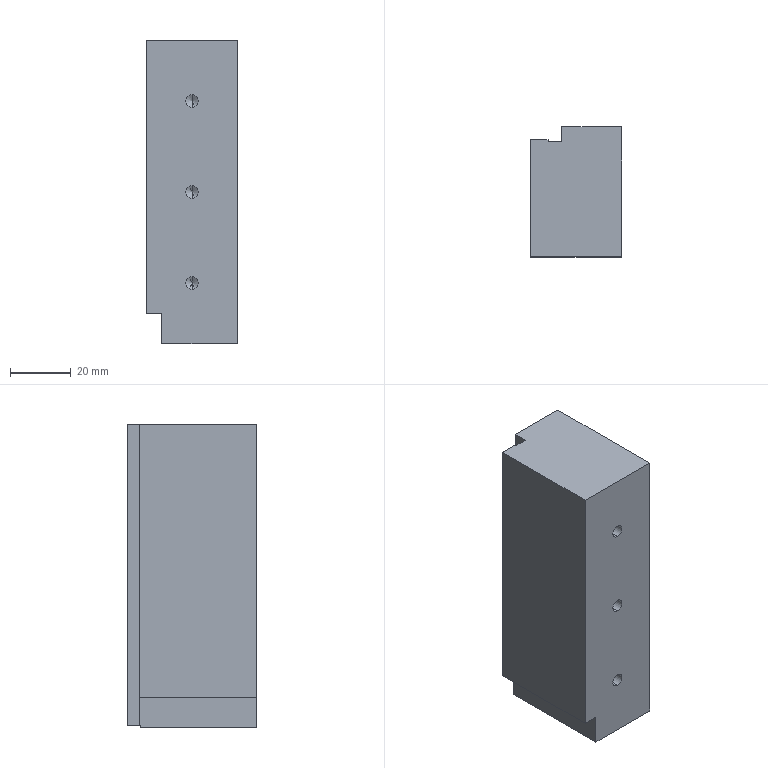Part | STEP file | Harpoon feed slide_Default | 1 solid | 52 faces | box 30 x 42.8 x 100 mm | volume 120679 mm3 | cylinder 18 | cone 18 | plane 16 | commonest cylinder face diameters 4.2 x10 2.5 x8